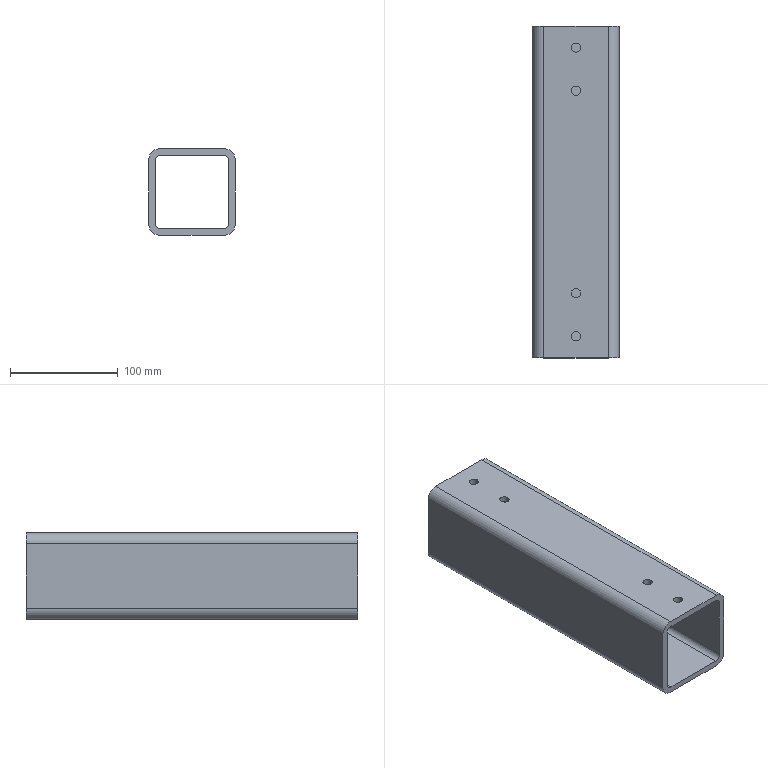Part | SolidWorks | features HoleWzd 3, Fillet 2, Extrusion 1, ICE 1 | 1 solid | 26 faces | box 80 x 307.64 x 80 mm | volume 500055 mm3 | cylinder 16 | plane 10 | commonest cylinder face diameters 8.5 x8 10 x4 20 x4
STEP:
#1=CARTESIAN_POINT('',(0.75,-1.503,34.3));
#2=VERTEX_POINT('',#1);
#3=CARTESIAN_POINT('',(9.25,-1.503,34.3));
#4=VERTEX_POINT('',#3);
#5=CARTESIAN_POINT('',(5.,-1.503,34.3));
#6=DIRECTION('',(0.,0.,1.));
#7=DIRECTION('',(1.,0.,0.));
#8=AXIS2_PLACEMENT_3D('',#5,#6,#7);
#9=CIRCLE('',#8,4.25);
#10=EDGE_CURVE('',#2,#4,#9,.T.);
#11=ORIENTED_EDGE('',*,*,#10,.F.);
#12=CARTESIAN_POINT('',(0.75,-1.503,40.));
#13=VERTEX_POINT('',#12);
#14=CARTESIAN_POINT('',(0.75,-1.503,40.));
#15=DIRECTION('',(0.,0.,1.));
#16=VECTOR('',#15,1000.);
#17=LINE('',#14,#16);
#18=EDGE_CURVE('',#2,#13,#17,.T.);
#19=ORIENTED_EDGE('',*,*,#18,.T.);
#20=CARTESIAN_POINT('',(9.25,-1.503,40.));
#21=VERTEX_POINT('',#20);
#22=CARTESIAN_POINT('',(5.,-1.503,40.));
#23=DIRECTION('',(0.,0.,1.));
#24=DIRECTION('',(1.,0.,0.));
#25=AXIS2_PLACEMENT_3D('',#22,#23,#24);
#26=CIRCLE('',#25,4.25);
#27=EDGE_CURVE('',#13,#21,#26,.T.);
#28=ORIENTED_EDGE('',*,*,#27,.T.);
#29=CARTESIAN_POINT('',(9.25,-1.503,40.));
#30=DIRECTION('',(0.,0.,1.));
#31=VECTOR('',#30,1000.);
#32=LINE('',#29,#31);
#33=EDGE_CURVE('',#4,#21,#32,.T.);
#34=ORIENTED_EDGE('',*,*,#33,.F.);
#35=EDGE_LOOP('',(#11,#19,#28,#34));
#36=FACE_OUTER_BOUND('',#35,.T.);
#37=CARTESIAN_POINT('',(5.,-1.503,40.));
#38=DIRECTION('',(0.,0.,1.));
#39=DIRECTION('',(1.,0.,0.));
#40=AXIS2_PLACEMENT_3D('',#37,#38,#39);
#41=CYLINDRICAL_SURFACE('',#40,4.25);
#42=ADVANCED_FACE('',(#36),#41,.F.);
#43=CARTESIAN_POINT('',(0.75,38.497,34.3));
#44=VERTEX_POINT('',#43);
#45=CARTESIAN_POINT('',(9.25,38.497,34.3));
#46=VERTEX_POINT('',#45);
#47=CARTESIAN_POINT('',(5.,38.497,34.3));
#48=DIRECTION('',(0.,0.,1.));
#49=DIRECTION('',(1.,0.,0.));
#50=AXIS2_PLACEMENT_3D('',#47,#48,#49);
#51=CIRCLE('',#50,4.25);
#52=EDGE_CURVE('',#44,#46,#51,.T.);
#53=ORIENTED_EDGE('',*,*,#52,.F.);
#54=CARTESIAN_POINT('',(0.75,38.497,40.));
#55=VERTEX_POINT('',#54);
#56=CARTESIAN_POINT('',(0.75,38.497,40.));
#57=DIRECTION('',(0.,0.,1.));
#58=VECTOR('',#57,1000.);
#59=LINE('',#56,#58);
#60=EDGE_CURVE('',#44,#55,#59,.T.);
#61=ORIENTED_EDGE('',*,*,#60,.T.);
#62=CARTESIAN_POINT('',(9.25,38.497,40.));
#63=VERTEX_POINT('',#62);
#64=CARTESIAN_POINT('',(5.,38.497,40.));
#65=DIRECTION('',(0.,0.,1.));
#66=DIRECTION('',(1.,0.,0.));
#67=AXIS2_PLACEMENT_3D('',#64,#65,#66);
#68=CIRCLE('',#67,4.25);
#69=EDGE_CURVE('',#55,#63,#68,.T.);
#70=ORIENTED_EDGE('',*,*,#69,.T.);
#71=CARTESIAN_POINT('',(9.25,38.497,40.));
#72=DIRECTION('',(0.,0.,1.));
#73=VECTOR('',#72,1000.);
#74=LINE('',#71,#73);
#75=EDGE_CURVE('',#46,#63,#74,.T.);
#76=ORIENTED_EDGE('',*,*,#75,.F.);
#77=EDGE_LOOP('',(#53,#61,#70,#76));
#78=FACE_OUTER_BOUND('',#77,.T.);
#79=CARTESIAN_POINT('',(5.,38.497,40.));
#80=DIRECTION('',(0.,0.,1.));
#81=DIRECTION('',(1.,0.,0.));
#82=AXIS2_PLACEMENT_3D('',#79,#80,#81);
#83=CYLINDRICAL_SURFACE('',#82,4.25);
#84=ADVANCED_FACE('',(#78),#83,.F.);
#85=CARTESIAN_POINT('',(0.75,-189.143,34.3));
#86=VERTEX_POINT('',#85);
#87=CARTESIAN_POINT('',(9.25,-189.143,34.3));
#88=VERTEX_POINT('',#87);
#89=CARTESIAN_POINT('',(5.,-189.143,34.3));
#90=DIRECTION('',(0.,0.,1.));
#91=DIRECTION('',(1.,0.,0.));
#92=AXIS2_PLACEMENT_3D('',#89,#90,#91);
#93=CIRCLE('',#92,4.25);
#94=EDGE_CURVE('',#86,#88,#93,.T.);
#95=ORIENTED_EDGE('',*,*,#94,.F.);
#96=CARTESIAN_POINT('',(0.75,-189.143,40.));
#97=VERTEX_POINT('',#96);
#98=CARTESIAN_POINT('',(0.75,-189.143,40.));
#99=DIRECTION('',(0.,0.,1.));
#100=VECTOR('',#99,1000.);
#101=LINE('',#98,#100);
#102=EDGE_CURVE('',#86,#97,#101,.T.);
#103=ORIENTED_EDGE('',*,*,#102,.T.);
#104=CARTESIAN_POINT('',(9.25,-189.143,40.));
#105=VERTEX_POINT('',#104);
#106=CARTESIAN_POINT('',(5.,-189.143,40.));
#107=DIRECTION('',(0.,0.,1.));
#108=DIRECTION('',(1.,0.,0.));
#109=AXIS2_PLACEMENT_3D('',#106,#107,#108);
#110=CIRCLE('',#109,4.25);
#111=EDGE_CURVE('',#97,#105,#110,.T.);
#112=ORIENTED_EDGE('',*,*,#111,.T.);
#113=CARTESIAN_POINT('',(9.25,-189.143,40.));
#114=DIRECTION('',(0.,0.,1.));
#115=VECTOR('',#114,1000.);
#116=LINE('',#113,#115);
#117=EDGE_CURVE('',#88,#105,#116,.T.);
#118=ORIENTED_EDGE('',*,*,#117,.F.);
#119=EDGE_LOOP('',(#95,#103,#112,#118));
#120=FACE_OUTER_BOUND('',#119,.T.);
#121=CARTESIAN_POINT('',(5.,-189.143,40.));
#122=DIRECTION('',(0.,0.,1.));
#123=DIRECTION('',(1.,0.,0.));
#124=AXIS2_PLACEMENT_3D('',#121,#122,#123);
#125=CYLINDRICAL_SURFACE('',#124,4.25);
#126=ADVANCED_FACE('',(#120),#125,.F.);
#127=CARTESIAN_POINT('',(0.75,-229.143,34.3));
#128=VERTEX_POINT('',#127);
#129=CARTESIAN_POINT('',(9.25,-229.143,34.3));
#130=VERTEX_POINT('',#129);
#131=CARTESIAN_POINT('',(5.,-229.143,34.3));
#132=DIRECTION('',(0.,0.,1.));
#133=DIRECTION('',(1.,0.,0.));
#134=AXIS2_PLACEMENT_3D('',#131,#132,#133);
#135=CIRCLE('',#134,4.25);
#136=EDGE_CURVE('',#128,#130,#135,.T.);
#137=ORIENTED_EDGE('',*,*,#136,.F.);
#138=CARTESIAN_POINT('',(0.75,-229.143,40.));
#139=VERTEX_POINT('',#138);
#140=CARTESIAN_POINT('',(0.75,-229.143,40.));
#141=DIRECTION('',(0.,0.,1.));
#142=VECTOR('',#141,1000.);
#143=LINE('',#140,#142);
#144=EDGE_CURVE('',#128,#139,#143,.T.);
#145=ORIENTED_EDGE('',*,*,#144,.T.);
#146=CARTESIAN_POINT('',(9.25,-229.143,40.));
#147=VERTEX_POINT('',#146);
#148=CARTESIAN_POINT('',(5.,-229.143,40.));
#149=DIRECTION('',(0.,0.,1.));
#150=DIRECTION('',(1.,0.,0.));
#151=AXIS2_PLACEMENT_3D('',#148,#149,#150);
#152=CIRCLE('',#151,4.25);
#153=EDGE_CURVE('',#139,#147,#152,.T.);
#154=ORIENTED_EDGE('',*,*,#153,.T.);
#155=CARTESIAN_POINT('',(9.25,-229.143,40.));
#156=DIRECTION('',(0.,0.,1.));
#157=VECTOR('',#156,1000.);
#158=LINE('',#155,#157);
#159=EDGE_CURVE('',#130,#147,#158,.T.);
#160=ORIENTED_EDGE('',*,*,#159,.F.);
#161=EDGE_LOOP('',(#137,#145,#154,#160));
#162=FACE_OUTER_BOUND('',#161,.T.);
#163=CARTESIAN_POINT('',(5.,-229.143,40.));
#164=DIRECTION('',(0.,0.,1.));
#165=DIRECTION('',(1.,0.,0.));
#166=AXIS2_PLACEMENT_3D('',#163,#164,#165);
#167=CYLINDRICAL_SURFACE('',#166,4.25);
#168=ADVANCED_FACE('',(#162),#167,.F.);
#169=CARTESIAN_POINT('',(35.,-249.143,-40.));
#170=VERTEX_POINT('',#169);
#171=CARTESIAN_POINT('',(-25.,-249.143,-40.));
#172=VERTEX_POINT('',#171);
#173=CARTESIAN_POINT('',(45.,-249.143,-40.));
#174=DIRECTION('',(-1.,0.,0.));
#175=VECTOR('',#174,1000.);
#176=LINE('',#173,#175);
#177=EDGE_CURVE('',#170,#172,#176,.T.);
#178=ORIENTED_EDGE('',*,*,#177,.T.);
#179=CARTESIAN_POINT('',(-25.,58.497,-40.));
#180=VERTEX_POINT('',#179);
#181=CARTESIAN_POINT('',(-25.,58.497,-40.));
#182=DIRECTION('',(0.,1.,0.));
#183=VECTOR('',#182,1000.);
#184=LINE('',#181,#183);
#185=EDGE_CURVE('',#172,#180,#184,.T.);
#186=ORIENTED_EDGE('',*,*,#185,.T.);
#187=CARTESIAN_POINT('',(35.,58.497,-40.));
#188=VERTEX_POINT('',#187);
#189=CARTESIAN_POINT('',(45.,58.497,-40.));
#190=DIRECTION('',(-1.,0.,0.));
#191=VECTOR('',#190,1000.);
#192=LINE('',#189,#191);
#193=EDGE_CURVE('',#188,#180,#192,.T.);
#194=ORIENTED_EDGE('',*,*,#193,.F.);
#195=CARTESIAN_POINT('',(35.,-249.143,-40.));
#196=DIRECTION('',(0.,-1.,0.));
#197=VECTOR('',#196,1000.);
#198=LINE('',#195,#197);
#199=EDGE_CURVE('',#188,#170,#198,.T.);
#200=ORIENTED_EDGE('',*,*,#199,.T.);
#201=EDGE_LOOP('',(#178,#186,#194,#200));
#202=FACE_OUTER_BOUND('',#201,.T.);
#203=CARTESIAN_POINT('',(45.,58.497,-40.));
#204=DIRECTION('',(0.,0.,-1.));
#205=DIRECTION('',(-1.,0.,0.));
#206=AXIS2_PLACEMENT_3D('',#203,#204,#205);
#207=PLANE('',#206);
#208=ADVANCED_FACE('',(#202),#207,.T.);
#209=CARTESIAN_POINT('',(34.3,58.497,34.3));
#210=VERTEX_POINT('',#209);
#211=CARTESIAN_POINT('',(-24.3,58.497,34.3));
#212=VERTEX_POINT('',#211);
#213=CARTESIAN_POINT('',(39.3,58.497,34.3));
#214=DIRECTION('',(-1.,0.,0.));
#215=VECTOR('',#214,1000.);
#216=LINE('',#213,#215);
#217=EDGE_CURVE('',#210,#212,#216,.T.);
#218=ORIENTED_EDGE('',*,*,#217,.T.);
#219=CARTESIAN_POINT('',(-29.3,58.497,29.3));
#220=VERTEX_POINT('',#219);
#221=CARTESIAN_POINT('',(-24.3,58.497,29.3));
#222=DIRECTION('',(0.,-1.,0.));
#223=DIRECTION('',(0.,0.,1.));
#224=AXIS2_PLACEMENT_3D('',#221,#222,#223);
#225=CIRCLE('',#224,5.);
#226=EDGE_CURVE('',#212,#220,#225,.T.);
#227=ORIENTED_EDGE('',*,*,#226,.T.);
#228=CARTESIAN_POINT('',(-29.3,58.497,-29.3));
#229=VERTEX_POINT('',#228);
#230=CARTESIAN_POINT('',(-29.3,58.497,34.3));
#231=DIRECTION('',(0.,0.,-1.));
#232=VECTOR('',#231,1000.);
#233=LINE('',#230,#232);
#234=EDGE_CURVE('',#220,#229,#233,.T.);
#235=ORIENTED_EDGE('',*,*,#234,.T.);
#236=CARTESIAN_POINT('',(-24.3,58.497,-34.3));
#237=VERTEX_POINT('',#236);
#238=CARTESIAN_POINT('',(-24.3,58.497,-29.3));
#239=DIRECTION('',(0.,-1.,0.));
#240=DIRECTION('',(0.,0.,1.));
#241=AXIS2_PLACEMENT_3D('',#238,#239,#240);
#242=CIRCLE('',#241,5.);
#243=EDGE_CURVE('',#229,#237,#242,.T.);
#244=ORIENTED_EDGE('',*,*,#243,.T.);
#245=CARTESIAN_POINT('',(34.3,58.497,-34.3));
#246=VERTEX_POINT('',#245);
#247=CARTESIAN_POINT('',(-29.3,58.497,-34.3));
#248=DIRECTION('',(1.,0.,0.));
#249=VECTOR('',#248,1000.);
#250=LINE('',#247,#249);
#251=EDGE_CURVE('',#237,#246,#250,.T.);
#252=ORIENTED_EDGE('',*,*,#251,.T.);
#253=CARTESIAN_POINT('',(39.3,58.497,-29.3));
#254=VERTEX_POINT('',#253);
#255=CARTESIAN_POINT('',(34.3,58.497,-29.3));
#256=DIRECTION('',(0.,-1.,0.));
#257=DIRECTION('',(0.,0.,1.));
#258=AXIS2_PLACEMENT_3D('',#255,#256,#257);
#259=CIRCLE('',#258,5.);
#260=EDGE_CURVE('',#246,#254,#259,.T.);
#261=ORIENTED_EDGE('',*,*,#260,.T.);
#262=CARTESIAN_POINT('',(39.3,58.497,29.3));
#263=VERTEX_POINT('',#262);
#264=CARTESIAN_POINT('',(39.3,58.497,-34.3));
#265=DIRECTION('',(0.,0.,1.));
#266=VECTOR('',#265,1000.);
#267=LINE('',#264,#266);
#268=EDGE_CURVE('',#254,#263,#267,.T.);
#269=ORIENTED_EDGE('',*,*,#268,.T.);
#270=CARTESIAN_POINT('',(34.3,58.497,29.3));
#271=DIRECTION('',(0.,-1.,0.));
#272=DIRECTION('',(0.,0.,1.));
#273=AXIS2_PLACEMENT_3D('',#270,#271,#272);
#274=CIRCLE('',#273,5.);
#275=EDGE_CURVE('',#263,#210,#274,.T.);
#276=ORIENTED_EDGE('',*,*,#275,.T.);
#277=EDGE_LOOP('',(#218,#227,#235,#244,#252,#261,#269,#276));
#278=FACE_BOUND('',#277,.T.);
#279=CARTESIAN_POINT('',(-35.,58.497,30.));
#280=VERTEX_POINT('',#279);
#281=CARTESIAN_POINT('',(-35.,58.497,-30.));
#282=VERTEX_POINT('',#281);
#283=CARTESIAN_POINT('',(-35.,58.497,40.));
#284=DIRECTION('',(0.,0.,-1.));
#285=VECTOR('',#284,1000.);
#286=LINE('',#283,#285);
#287=EDGE_CURVE('',#280,#282,#286,.T.);
#288=ORIENTED_EDGE('',*,*,#287,.F.);
#289=CARTESIAN_POINT('',(-25.,58.497,40.));
#290=VERTEX_POINT('',#289);
#291=CARTESIAN_POINT('',(-25.,58.497,30.));
#292=DIRECTION('',(0.,1.,0.));
#293=DIRECTION('',(0.,0.,1.));
#294=AXIS2_PLACEMENT_3D('',#291,#292,#293);
#295=CIRCLE('',#294,10.);
#296=EDGE_CURVE('',#280,#290,#295,.T.);
#297=ORIENTED_EDGE('',*,*,#296,.T.);
#298=CARTESIAN_POINT('',(35.,58.497,40.));
#299=VERTEX_POINT('',#298);
#300=CARTESIAN_POINT('',(45.,58.497,40.));
#301=DIRECTION('',(-1.,0.,0.));
#302=VECTOR('',#301,1000.);
#303=LINE('',#300,#302);
#304=EDGE_CURVE('',#299,#290,#303,.T.);
#305=ORIENTED_EDGE('',*,*,#304,.F.);
#306=CARTESIAN_POINT('',(45.,58.497,30.));
#307=VERTEX_POINT('',#306);
#308=CARTESIAN_POINT('',(35.,58.497,30.));
#309=DIRECTION('',(0.,1.,0.));
#310=DIRECTION('',(0.,0.,1.));
#311=AXIS2_PLACEMENT_3D('',#308,#309,#310);
#312=CIRCLE('',#311,10.);
#313=EDGE_CURVE('',#299,#307,#312,.T.);
#314=ORIENTED_EDGE('',*,*,#313,.T.);
#315=CARTESIAN_POINT('',(45.,58.497,-30.));
#316=VERTEX_POINT('',#315);
#317=CARTESIAN_POINT('',(45.,58.497,40.));
#318=DIRECTION('',(0.,0.,-1.));
#319=VECTOR('',#318,1000.);
#320=LINE('',#317,#319);
#321=EDGE_CURVE('',#307,#316,#320,.T.);
#322=ORIENTED_EDGE('',*,*,#321,.T.);
#323=CARTESIAN_POINT('',(35.,58.497,-30.));
#324=DIRECTION('',(0.,1.,0.));
#325=DIRECTION('',(0.,0.,1.));
#326=AXIS2_PLACEMENT_3D('',#323,#324,#325);
#327=CIRCLE('',#326,10.);
#328=EDGE_CURVE('',#316,#188,#327,.T.);
#329=ORIENTED_EDGE('',*,*,#328,.T.);
#330=ORIENTED_EDGE('',*,*,#193,.T.);
#331=CARTESIAN_POINT('',(-25.,58.497,-30.));
#332=DIRECTION('',(0.,1.,0.));
#333=DIRECTION('',(0.,0.,1.));
#334=AXIS2_PLACEMENT_3D('',#331,#332,#333);
#335=CIRCLE('',#334,10.);
#336=EDGE_CURVE('',#180,#282,#335,.T.);
#337=ORIENTED_EDGE('',*,*,#336,.T.);
#338=EDGE_LOOP('',(#288,#297,#305,#314,#322,#329,#330,#337));
#339=FACE_OUTER_BOUND('',#338,.T.);
#340=CARTESIAN_POINT('',(45.,58.497,40.));
#341=DIRECTION('',(0.,1.,0.));
#342=DIRECTION('',(0.,0.,1.));
#343=AXIS2_PLACEMENT_3D('',#340,#341,#342);
#344=PLANE('',#343);
#345=ADVANCED_FACE('',(#278,#339),#344,.T.);
#346=CARTESIAN_POINT('',(5.,-1.503,40.));
#347=DIRECTION('',(0.,0.,1.));
#348=DIRECTION('',(1.,0.,0.));
#349=AXIS2_PLACEMENT_3D('',#346,#347,#348);
#350=CIRCLE('',#349,4.25);
#351=EDGE_CURVE('',#21,#13,#350,.T.);
#352=ORIENTED_EDGE('',*,*,#351,.F.);
#353=ORIENTED_EDGE('',*,*,#27,.F.);
#354=EDGE_LOOP('',(#352,#353));
#355=FACE_BOUND('',#354,.T.);
#356=CARTESIAN_POINT('',(5.,38.497,40.));
#357=DIRECTION('',(0.,0.,1.));
#358=DIRECTION('',(1.,0.,0.));
#359=AXIS2_PLACEMENT_3D('',#356,#357,#358);
#360=CIRCLE('',#359,4.25);
#361=EDGE_CURVE('',#63,#55,#360,.T.);
#362=ORIENTED_EDGE('',*,*,#361,.F.);
#363=ORIENTED_EDGE('',*,*,#69,.F.);
#364=EDGE_LOOP('',(#362,#363));
#365=FACE_BOUND('',#364,.T.);
#366=CARTESIAN_POINT('',(5.,-189.143,40.));
#367=DIRECTION('',(0.,0.,1.));
#368=DIRECTION('',(1.,0.,0.));
#369=AXIS2_PLACEMENT_3D('',#366,#367,#368);
#370=CIRCLE('',#369,4.25);
#371=EDGE_CURVE('',#105,#97,#370,.T.);
#372=ORIENTED_EDGE('',*,*,#371,.F.);
#373=ORIENTED_EDGE('',*,*,#111,.F.);
#374=EDGE_LOOP('',(#372,#373));
#375=FACE_BOUND('',#374,.T.);
#376=CARTESIAN_POINT('',(5.,-229.143,40.));
#377=DIRECTION('',(0.,0.,1.));
#378=DIRECTION('',(1.,0.,0.));
#379=AXIS2_PLACEMENT_3D('',#376,#377,#378);
#380=CIRCLE('',#379,4.25);
#381=EDGE_CURVE('',#147,#139,#380,.T.);
#382=ORIENTED_EDGE('',*,*,#381,.F.);
#383=ORIENTED_EDGE('',*,*,#153,.F.);
#384=EDGE_LOOP('',(#382,#383));
#385=FACE_BOUND('',#384,.T.);
#386=ORIENTED_EDGE('',*,*,#304,.T.);
#387=CARTESIAN_POINT('',(-25.,-249.143,40.));
#388=VERTEX_POINT('',#387);
#389=CARTESIAN_POINT('',(-25.,-249.143,40.));
#390=DIRECTION('',(0.,-1.,0.));
#391=VECTOR('',#390,1000.);
#392=LINE('',#389,#391);
#393=EDGE_CURVE('',#290,#388,#392,.T.);
#394=ORIENTED_EDGE('',*,*,#393,.T.);
#395=CARTESIAN_POINT('',(35.,-249.143,40.));
#396=VERTEX_POINT('',#395);
#397=CARTESIAN_POINT('',(45.,-249.143,40.));
#398=DIRECTION('',(-1.,0.,0.));
#399=VECTOR('',#398,1000.);
#400=LINE('',#397,#399);
#401=EDGE_CURVE('',#396,#388,#400,.T.);
#402=ORIENTED_EDGE('',*,*,#401,.F.);
#403=CARTESIAN_POINT('',(35.,58.497,40.));
#404=DIRECTION('',(0.,1.,0.));
#405=VECTOR('',#404,1000.);
#406=LINE('',#403,#405);
#407=EDGE_CURVE('',#396,#299,#406,.T.);
#408=ORIENTED_EDGE('',*,*,#407,.T.);
#409=EDGE_LOOP('',(#386,#394,#402,#408));
#410=FACE_OUTER_BOUND('',#409,.T.);
#411=CARTESIAN_POINT('',(45.,-249.143,40.));
#412=DIRECTION('',(0.,0.,1.));
#413=DIRECTION('',(0.,-1.,0.));
#414=AXIS2_PLACEMENT_3D('',#411,#412,#413);
#415=PLANE('',#414);
#416=ADVANCED_FACE('',(#355,#365,#375,#385,#410),#415,.T.);
#417=CARTESIAN_POINT('',(-29.3,-249.143,29.3));
#418=VERTEX_POINT('',#417);
#419=CARTESIAN_POINT('',(-29.3,-249.143,-29.3));
#420=VERTEX_POINT('',#419);
#421=CARTESIAN_POINT('',(-29.3,-249.143,34.3));
#422=DIRECTION('',(0.,0.,-1.));
#423=VECTOR('',#422,1000.);
#424=LINE('',#421,#423);
#425=EDGE_CURVE('',#418,#420,#424,.T.);
#426=ORIENTED_EDGE('',*,*,#425,.F.);
#427=CARTESIAN_POINT('',(-24.3,-249.143,34.3));
#428=VERTEX_POINT('',#427);
#429=CARTESIAN_POINT('',(-24.3,-249.143,29.3));
#430=DIRECTION('',(0.,1.,0.));
#431=DIRECTION('',(0.,0.,-1.));
#432=AXIS2_PLACEMENT_3D('',#429,#430,#431);
#433=CIRCLE('',#432,5.);
#434=EDGE_CURVE('',#418,#428,#433,.T.);
#435=ORIENTED_EDGE('',*,*,#434,.T.);
#436=CARTESIAN_POINT('',(34.3,-249.143,34.3));
#437=VERTEX_POINT('',#436);
#438=CARTESIAN_POINT('',(39.3,-249.143,34.3));
#439=DIRECTION('',(-1.,0.,0.));
#440=VECTOR('',#439,1000.);
#441=LINE('',#438,#440);
#442=EDGE_CURVE('',#437,#428,#441,.T.);
#443=ORIENTED_EDGE('',*,*,#442,.F.);
#444=CARTESIAN_POINT('',(39.3,-249.143,29.3));
#445=VERTEX_POINT('',#444);
#446=CARTESIAN_POINT('',(34.3,-249.143,29.3));
#447=DIRECTION('',(0.,1.,0.));
#448=DIRECTION('',(0.,0.,-1.));
#449=AXIS2_PLACEMENT_3D('',#446,#447,#448);
#450=CIRCLE('',#449,5.);
#451=EDGE_CURVE('',#437,#445,#450,.T.);
#452=ORIENTED_EDGE('',*,*,#451,.T.);
#453=CARTESIAN_POINT('',(39.3,-249.143,-29.3));
#454=VERTEX_POINT('',#453);
#455=CARTESIAN_POINT('',(39.3,-249.143,-34.3));
#456=DIRECTION('',(0.,0.,1.));
#457=VECTOR('',#456,1000.);
#458=LINE('',#455,#457);
#459=EDGE_CURVE('',#454,#445,#458,.T.);
#460=ORIENTED_EDGE('',*,*,#459,.F.);
#461=CARTESIAN_POINT('',(34.3,-249.143,-34.3));
#462=VERTEX_POINT('',#461);
#463=CARTESIAN_POINT('',(34.3,-249.143,-29.3));
#464=DIRECTION('',(0.,1.,0.));
#465=DIRECTION('',(0.,0.,-1.));
#466=AXIS2_PLACEMENT_3D('',#463,#464,#465);
#467=CIRCLE('',#466,5.);
#468=EDGE_CURVE('',#454,#462,#467,.T.);
#469=ORIENTED_EDGE('',*,*,#468,.T.);
#470=CARTESIAN_POINT('',(-24.3,-249.143,-34.3));
#471=VERTEX_POINT('',#470);
#472=CARTESIAN_POINT('',(-29.3,-249.143,-34.3));
#473=DIRECTION('',(1.,0.,0.));
#474=VECTOR('',#473,1000.);
#475=LINE('',#472,#474);
#476=EDGE_CURVE('',#471,#462,#475,.T.);
#477=ORIENTED_EDGE('',*,*,#476,.F.);
#478=CARTESIAN_POINT('',(-24.3,-249.143,-29.3));
#479=DIRECTION('',(0.,1.,0.));
#480=DIRECTION('',(0.,0.,-1.));
#481=AXIS2_PLACEMENT_3D('',#478,#479,#480);
#482=CIRCLE('',#481,5.);
#483=EDGE_CURVE('',#471,#420,#482,.T.);
#484=ORIENTED_EDGE('',*,*,#483,.T.);
#485=EDGE_LOOP('',(#426,#435,#443,#452,#460,#469,#477,#484));
#486=FACE_BOUND('',#485,.T.);
#487=ORIENTED_EDGE('',*,*,#401,.T.);
#488=CARTESIAN_POINT('',(-35.,-249.143,30.));
#489=VERTEX_POINT('',#488);
#490=CARTESIAN_POINT('',(-25.,-249.143,30.));
#491=DIRECTION('',(0.,-1.,0.));
#492=DIRECTION('',(0.,0.,-1.));
#493=AXIS2_PLACEMENT_3D('',#490,#491,#492);
#494=CIRCLE('',#493,10.);
#495=EDGE_CURVE('',#388,#489,#494,.T.);
#496=ORIENTED_EDGE('',*,*,#495,.T.);
#497=CARTESIAN_POINT('',(-35.,-249.143,-30.));
#498=VERTEX_POINT('',#497);
#499=CARTESIAN_POINT('',(-35.,-249.143,-40.));
#500=DIRECTION('',(0.,0.,1.));
#501=VECTOR('',#500,1000.);
#502=LINE('',#499,#501);
#503=EDGE_CURVE('',#498,#489,#502,.T.);
#504=ORIENTED_EDGE('',*,*,#503,.F.);
#505=CARTESIAN_POINT('',(-25.,-249.143,-30.));
#506=DIRECTION('',(0.,-1.,0.));
#507=DIRECTION('',(0.,0.,-1.));
#508=AXIS2_PLACEMENT_3D('',#505,#506,#507);
#509=CIRCLE('',#508,10.);
#510=EDGE_CURVE('',#498,#172,#509,.T.);
#511=ORIENTED_EDGE('',*,*,#510,.T.);
#512=ORIENTED_EDGE('',*,*,#177,.F.);
#513=CARTESIAN_POINT('',(45.,-249.143,-30.));
#514=VERTEX_POINT('',#513);
#515=CARTESIAN_POINT('',(35.,-249.143,-30.));
#516=DIRECTION('',(0.,-1.,0.));
#517=DIRECTION('',(0.,0.,-1.));
#518=AXIS2_PLACEMENT_3D('',#515,#516,#517);
#519=CIRCLE('',#518,10.);
#520=EDGE_CURVE('',#170,#514,#519,.T.);
#521=ORIENTED_EDGE('',*,*,#520,.T.);
#522=CARTESIAN_POINT('',(45.,-249.143,30.));
#523=VERTEX_POINT('',#522);
#524=CARTESIAN_POINT('',(45.,-249.143,-40.));
#525=DIRECTION('',(0.,0.,1.));
#526=VECTOR('',#525,1000.);
#527=LINE('',#524,#526);
#528=EDGE_CURVE('',#514,#523,#527,.T.);
#529=ORIENTED_EDGE('',*,*,#528,.T.);
#530=CARTESIAN_POINT('',(35.,-249.143,30.));
#531=DIRECTION('',(0.,-1.,0.));
#532=DIRECTION('',(0.,0.,-1.));
#533=AXIS2_PLACEMENT_3D('',#530,#531,#532);
#534=CIRCLE('',#533,10.);
#535=EDGE_CURVE('',#523,#396,#534,.T.);
#536=ORIENTED_EDGE('',*,*,#535,.T.);
#537=EDGE_LOOP('',(#487,#496,#504,#511,#512,#521,#529,#536));
#538=FACE_OUTER_BOUND('',#537,.T.);
#539=CARTESIAN_POINT('',(45.,-249.143,-40.));
#540=DIRECTION('',(0.,-1.,0.));
#541=DIRECTION('',(0.,0.,-1.));
#542=AXIS2_PLACEMENT_3D('',#539,#540,#541);
#543=PLANE('',#542);
#544=ADVANCED_FACE('',(#486,#538),#543,.T.);
#545=ORIENTED_EDGE('',*,*,#321,.F.);
#546=CARTESIAN_POINT('',(45.,-249.143,30.));
#547=DIRECTION('',(0.,-1.,0.));
#548=VECTOR('',#547,1000.);
#549=LINE('',#546,#548);
#550=EDGE_CURVE('',#307,#523,#549,.T.);
#551=ORIENTED_EDGE('',*,*,#550,.T.);
#552=ORIENTED_EDGE('',*,*,#528,.F.);
#553=CARTESIAN_POINT('',(45.,58.497,-30.));
#554=DIRECTION('',(0.,1.,0.));
#555=VECTOR('',#554,1000.);
#556=LINE('',#553,#555);
#557=EDGE_CURVE('',#514,#316,#556,.T.);
#558=ORIENTED_EDGE('',*,*,#557,.T.);
#559=EDGE_LOOP('',(#545,#551,#552,#558));
#560=FACE_OUTER_BOUND('',#559,.T.);
#561=CARTESIAN_POINT('',(45.,0.,0.));
#562=DIRECTION('',(-1.,0.,0.));
#563=DIRECTION('',(0.,0.,1.));
#564=AXIS2_PLACEMENT_3D('',#561,#562,#563);
#565=PLANE('',#564);
#566=ADVANCED_FACE('',(#560),#565,.F.);
#567=ORIENTED_EDGE('',*,*,#503,.T.);
#568=CARTESIAN_POINT('',(-35.,0.,30.));
#569=DIRECTION('',(0.,1.,0.));
#570=VECTOR('',#569,1000.);
#571=LINE('',#568,#570);
#572=EDGE_CURVE('',#489,#280,#571,.T.);
#573=ORIENTED_EDGE('',*,*,#572,.T.);
#574=ORIENTED_EDGE('',*,*,#287,.T.);
#575=CARTESIAN_POINT('',(-35.,0.,-30.));
#576=DIRECTION('',(0.,-1.,0.));
#577=VECTOR('',#576,1000.);
#578=LINE('',#575,#577);
#579=EDGE_CURVE('',#282,#498,#578,.T.);
#580=ORIENTED_EDGE('',*,*,#579,.T.);
#581=EDGE_LOOP('',(#567,#573,#574,#580));
#582=FACE_OUTER_BOUND('',#581,.T.);
#583=CARTESIAN_POINT('',(-35.,0.,0.));
#584=DIRECTION('',(-1.,0.,0.));
#585=DIRECTION('',(0.,0.,1.));
#586=AXIS2_PLACEMENT_3D('',#583,#584,#585);
#587=PLANE('',#586);
#588=ADVANCED_FACE('',(#582),#587,.T.);
#589=ORIENTED_EDGE('',*,*,#234,.F.);
#590=CARTESIAN_POINT('',(-29.3,-249.143,29.3));
#591=DIRECTION('',(0.,-1.,0.));
#592=VECTOR('',#591,1000.);
#593=LINE('',#590,#592);
#594=EDGE_CURVE('',#220,#418,#593,.T.);
#595=ORIENTED_EDGE('',*,*,#594,.T.);
#596=ORIENTED_EDGE('',*,*,#425,.T.);
#597=CARTESIAN_POINT('',(-29.3,58.497,-29.3));
#598=DIRECTION('',(0.,1.,0.));
#599=VECTOR('',#598,1000.);
#600=LINE('',#597,#599);
#601=EDGE_CURVE('',#420,#229,#600,.T.);
#602=ORIENTED_EDGE('',*,*,#601,.T.);
#603=EDGE_LOOP('',(#589,#595,#596,#602));
#604=FACE_OUTER_BOUND('',#603,.T.);
#605=CARTESIAN_POINT('',(-29.3,58.497,34.3));
#606=DIRECTION('',(-1.,0.,0.));
#607=DIRECTION('',(0.,0.,1.));
#608=AXIS2_PLACEMENT_3D('',#605,#606,#607);
#609=PLANE('',#608);
#610=ADVANCED_FACE('',(#604),#609,.F.);
#611=CARTESIAN_POINT('',(5.,-1.503,34.3));
#612=DIRECTION('',(0.,0.,1.));
#613=DIRECTION('',(1.,0.,0.));
#614=AXIS2_PLACEMENT_3D('',#611,#612,#613);
#615=CIRCLE('',#614,4.25);
#616=EDGE_CURVE('',#4,#2,#615,.T.);
#617=ORIENTED_EDGE('',*,*,#616,.T.);
#618=ORIENTED_EDGE('',*,*,#10,.T.);
#619=EDGE_LOOP('',(#617,#618));
#620=FACE_BOUND('',#619,.T.);
#621=CARTESIAN_POINT('',(5.,38.497,34.3));
#622=DIRECTION('',(0.,0.,1.));
#623=DIRECTION('',(1.,0.,0.));
#624=AXIS2_PLACEMENT_3D('',#621,#622,#623);
#625=CIRCLE('',#624,4.25);
#626=EDGE_CURVE('',#46,#44,#625,.T.);
#627=ORIENTED_EDGE('',*,*,#626,.T.);
#628=ORIENTED_EDGE('',*,*,#52,.T.);
#629=EDGE_LOOP('',(#627,#628));
#630=FACE_BOUND('',#629,.T.);
#631=CARTESIAN_POINT('',(5.,-189.143,34.3));
#632=DIRECTION('',(0.,0.,1.));
#633=DIRECTION('',(1.,0.,0.));
#634=AXIS2_PLACEMENT_3D('',#631,#632,#633);
#635=CIRCLE('',#634,4.25);
#636=EDGE_CURVE('',#88,#86,#635,.T.);
#637=ORIENTED_EDGE('',*,*,#636,.T.);
#638=ORIENTED_EDGE('',*,*,#94,.T.);
#639=EDGE_LOOP('',(#637,#638));
#640=FACE_BOUND('',#639,.T.);
#641=CARTESIAN_POINT('',(5.,-229.143,34.3));
#642=DIRECTION('',(0.,0.,1.));
#643=DIRECTION('',(1.,0.,0.));
#644=AXIS2_PLACEMENT_3D('',#641,#642,#643);
#645=CIRCLE('',#644,4.25);
#646=EDGE_CURVE('',#130,#128,#645,.T.);
#647=ORIENTED_EDGE('',*,*,#646,.T.);
#648=ORIENTED_EDGE('',*,*,#136,.T.);
#649=EDGE_LOOP('',(#647,#648));
#650=FACE_BOUND('',#649,.T.);
#651=ORIENTED_EDGE('',*,*,#217,.F.);
#652=CARTESIAN_POINT('',(34.3,-249.143,34.3));
#653=DIRECTION('',(0.,-1.,0.));
#654=VECTOR('',#653,1000.);
#655=LINE('',#652,#654);
#656=EDGE_CURVE('',#210,#437,#655,.T.);
#657=ORIENTED_EDGE('',*,*,#656,.T.);
#658=ORIENTED_EDGE('',*,*,#442,.T.);
#659=CARTESIAN_POINT('',(-24.3,58.497,34.3));
#660=DIRECTION('',(0.,1.,0.));
#661=VECTOR('',#660,1000.);
#662=LINE('',#659,#661);
#663=EDGE_CURVE('',#428,#212,#662,.T.);
#664=ORIENTED_EDGE('',*,*,#663,.T.);
#665=EDGE_LOOP('',(#651,#657,#658,#664));
#666=FACE_OUTER_BOUND('',#665,.T.);
#667=CARTESIAN_POINT('',(39.3,58.497,34.3));
#668=DIRECTION('',(0.,0.,1.));
#669=DIRECTION('',(1.,0.,0.));
#670=AXIS2_PLACEMENT_3D('',#667,#668,#669);
#671=PLANE('',#670);
#672=ADVANCED_FACE('',(#620,#630,#640,#650,#666),#671,.F.);
#673=ORIENTED_EDGE('',*,*,#459,.T.);
#674=CARTESIAN_POINT('',(39.3,58.497,29.3));
#675=DIRECTION('',(0.,1.,0.));
#676=VECTOR('',#675,1000.);
#677=LINE('',#674,#676);
#678=EDGE_CURVE('',#445,#263,#677,.T.);
#679=ORIENTED_EDGE('',*,*,#678,.T.);
#680=ORIENTED_EDGE('',*,*,#268,.F.);
#681=CARTESIAN_POINT('',(39.3,-249.143,-29.3));
#682=DIRECTION('',(0.,-1.,0.));
#683=VECTOR('',#682,1000.);
#684=LINE('',#681,#683);
#685=EDGE_CURVE('',#254,#454,#684,.T.);
#686=ORIENTED_EDGE('',*,*,#685,.T.);
#687=EDGE_LOOP('',(#673,#679,#680,#686));
#688=FACE_OUTER_BOUND('',#687,.T.);
#689=CARTESIAN_POINT('',(39.3,58.497,-34.3));
#690=DIRECTION('',(1.,0.,0.));
#691=DIRECTION('',(0.,0.,-1.));
#692=AXIS2_PLACEMENT_3D('',#689,#690,#691);
#693=PLANE('',#692);
#694=ADVANCED_FACE('',(#688),#693,.F.);
#695=ORIENTED_EDGE('',*,*,#476,.T.);
#696=CARTESIAN_POINT('',(34.3,58.497,-34.3));
#697=DIRECTION('',(0.,1.,0.));
#698=VECTOR('',#697,1000.);
#699=LINE('',#696,#698);
#700=EDGE_CURVE('',#462,#246,#699,.T.);
#701=ORIENTED_EDGE('',*,*,#700,.T.);
#702=ORIENTED_EDGE('',*,*,#251,.F.);
#703=CARTESIAN_POINT('',(-24.3,-249.143,-34.3));
#704=DIRECTION('',(0.,-1.,0.));
#705=VECTOR('',#704,1000.);
#706=LINE('',#703,#705);
#707=EDGE_CURVE('',#237,#471,#706,.T.);
#708=ORIENTED_EDGE('',*,*,#707,.T.);
#709=EDGE_LOOP('',(#695,#701,#702,#708));
#710=FACE_OUTER_BOUND('',#709,.T.);
#711=CARTESIAN_POINT('',(-29.3,58.497,-34.3));
#712=DIRECTION('',(0.,0.,-1.));
#713=DIRECTION('',(-1.,0.,0.));
#714=AXIS2_PLACEMENT_3D('',#711,#712,#713);
#715=PLANE('',#714);
#716=ADVANCED_FACE('',(#710),#715,.F.);
#717=ORIENTED_EDGE('',*,*,#144,.F.);
#718=ORIENTED_EDGE('',*,*,#646,.F.);
#719=ORIENTED_EDGE('',*,*,#159,.T.);
#720=ORIENTED_EDGE('',*,*,#381,.T.);
#721=EDGE_LOOP('',(#717,#718,#719,#720));
#722=FACE_OUTER_BOUND('',#721,.T.);
#723=CARTESIAN_POINT('',(5.,-229.143,40.));
#724=DIRECTION('',(0.,0.,1.));
#725=DIRECTION('',(1.,0.,0.));
#726=AXIS2_PLACEMENT_3D('',#723,#724,#725);
#727=CYLINDRICAL_SURFACE('',#726,4.25);
#728=ADVANCED_FACE('',(#722),#727,.F.);
#729=ORIENTED_EDGE('',*,*,#102,.F.);
#730=ORIENTED_EDGE('',*,*,#636,.F.);
#731=ORIENTED_EDGE('',*,*,#117,.T.);
#732=ORIENTED_EDGE('',*,*,#371,.T.);
#733=EDGE_LOOP('',(#729,#730,#731,#732));
#734=FACE_OUTER_BOUND('',#733,.T.);
#735=CARTESIAN_POINT('',(5.,-189.143,40.));
#736=DIRECTION('',(0.,0.,1.));
#737=DIRECTION('',(1.,0.,0.));
#738=AXIS2_PLACEMENT_3D('',#735,#736,#737);
#739=CYLINDRICAL_SURFACE('',#738,4.25);
#740=ADVANCED_FACE('',(#734),#739,.F.);
#741=ORIENTED_EDGE('',*,*,#275,.F.);
#742=ORIENTED_EDGE('',*,*,#678,.F.);
#743=ORIENTED_EDGE('',*,*,#451,.F.);
#744=ORIENTED_EDGE('',*,*,#656,.F.);
#745=EDGE_LOOP('',(#741,#742,#743,#744));
#746=FACE_OUTER_BOUND('',#745,.T.);
#747=CARTESIAN_POINT('',(34.3,58.497,29.3));
#748=DIRECTION('',(0.,1.,0.));
#749=DIRECTION('',(0.,0.,1.));
#750=AXIS2_PLACEMENT_3D('',#747,#748,#749);
#751=CYLINDRICAL_SURFACE('',#750,5.);
#752=ADVANCED_FACE('',(#746),#751,.F.);
#753=ORIENTED_EDGE('',*,*,#226,.F.);
#754=ORIENTED_EDGE('',*,*,#663,.F.);
#755=ORIENTED_EDGE('',*,*,#434,.F.);
#756=ORIENTED_EDGE('',*,*,#594,.F.);
#757=EDGE_LOOP('',(#753,#754,#755,#756));
#758=FACE_OUTER_BOUND('',#757,.T.);
#759=CARTESIAN_POINT('',(-24.3,58.497,29.3));
#760=DIRECTION('',(0.,1.,0.));
#761=DIRECTION('',(0.,0.,1.));
#762=AXIS2_PLACEMENT_3D('',#759,#760,#761);
#763=CYLINDRICAL_SURFACE('',#762,5.);
#764=ADVANCED_FACE('',(#758),#763,.F.);
#765=ORIENTED_EDGE('',*,*,#260,.F.);
#766=ORIENTED_EDGE('',*,*,#700,.F.);
#767=ORIENTED_EDGE('',*,*,#468,.F.);
#768=ORIENTED_EDGE('',*,*,#685,.F.);
#769=EDGE_LOOP('',(#765,#766,#767,#768));
#770=FACE_OUTER_BOUND('',#769,.T.);
#771=CARTESIAN_POINT('',(34.3,58.497,-29.3));
#772=DIRECTION('',(0.,1.,0.));
#773=DIRECTION('',(0.,0.,1.));
#774=AXIS2_PLACEMENT_3D('',#771,#772,#773);
#775=CYLINDRICAL_SURFACE('',#774,5.);
#776=ADVANCED_FACE('',(#770),#775,.F.);
#777=ORIENTED_EDGE('',*,*,#243,.F.);
#778=ORIENTED_EDGE('',*,*,#601,.F.);
#779=ORIENTED_EDGE('',*,*,#483,.F.);
#780=ORIENTED_EDGE('',*,*,#707,.F.);
#781=EDGE_LOOP('',(#777,#778,#779,#780));
#782=FACE_OUTER_BOUND('',#781,.T.);
#783=CARTESIAN_POINT('',(-24.3,58.497,-29.3));
#784=DIRECTION('',(0.,1.,0.));
#785=DIRECTION('',(0.,0.,1.));
#786=AXIS2_PLACEMENT_3D('',#783,#784,#785);
#787=CYLINDRICAL_SURFACE('',#786,5.);
#788=ADVANCED_FACE('',(#782),#787,.F.);
#789=ORIENTED_EDGE('',*,*,#495,.F.);
#790=ORIENTED_EDGE('',*,*,#393,.F.);
#791=ORIENTED_EDGE('',*,*,#296,.F.);
#792=ORIENTED_EDGE('',*,*,#572,.F.);
#793=EDGE_LOOP('',(#789,#790,#791,#792));
#794=FACE_OUTER_BOUND('',#793,.T.);
#795=CARTESIAN_POINT('',(-25.,0.,30.));
#796=DIRECTION('',(0.,1.,0.));
#797=DIRECTION('',(0.,0.,1.));
#798=AXIS2_PLACEMENT_3D('',#795,#796,#797);
#799=CYLINDRICAL_SURFACE('',#798,10.);
#800=ADVANCED_FACE('',(#794),#799,.T.);
#801=ORIENTED_EDGE('',*,*,#336,.F.);
#802=ORIENTED_EDGE('',*,*,#185,.F.);
#803=ORIENTED_EDGE('',*,*,#510,.F.);
#804=ORIENTED_EDGE('',*,*,#579,.F.);
#805=EDGE_LOOP('',(#801,#802,#803,#804));
#806=FACE_OUTER_BOUND('',#805,.T.);
#807=CARTESIAN_POINT('',(-25.,0.,-30.));
#808=DIRECTION('',(0.,-1.,0.));
#809=DIRECTION('',(0.,0.,-1.));
#810=AXIS2_PLACEMENT_3D('',#807,#808,#809);
#811=CYLINDRICAL_SURFACE('',#810,10.);
#812=ADVANCED_FACE('',(#806),#811,.T.);
#813=ORIENTED_EDGE('',*,*,#535,.F.);
#814=ORIENTED_EDGE('',*,*,#550,.F.);
#815=ORIENTED_EDGE('',*,*,#313,.F.);
#816=ORIENTED_EDGE('',*,*,#407,.F.);
#817=EDGE_LOOP('',(#813,#814,#815,#816));
#818=FACE_OUTER_BOUND('',#817,.T.);
#819=CARTESIAN_POINT('',(35.,-249.143,30.));
#820=DIRECTION('',(0.,-1.,0.));
#821=DIRECTION('',(0.,0.,-1.));
#822=AXIS2_PLACEMENT_3D('',#819,#820,#821);
#823=CYLINDRICAL_SURFACE('',#822,10.);
#824=ADVANCED_FACE('',(#818),#823,.T.);
#825=ORIENTED_EDGE('',*,*,#328,.F.);
#826=ORIENTED_EDGE('',*,*,#557,.F.);
#827=ORIENTED_EDGE('',*,*,#520,.F.);
#828=ORIENTED_EDGE('',*,*,#199,.F.);
#829=EDGE_LOOP('',(#825,#826,#827,#828));
#830=FACE_OUTER_BOUND('',#829,.T.);
#831=CARTESIAN_POINT('',(35.,58.497,-30.));
#832=DIRECTION('',(0.,1.,0.));
#833=DIRECTION('',(0.,0.,1.));
#834=AXIS2_PLACEMENT_3D('',#831,#832,#833);
#835=CYLINDRICAL_SURFACE('',#834,10.);
#836=ADVANCED_FACE('',(#830),#835,.T.);
#837=ORIENTED_EDGE('',*,*,#60,.F.);
#838=ORIENTED_EDGE('',*,*,#626,.F.);
#839=ORIENTED_EDGE('',*,*,#75,.T.);
#840=ORIENTED_EDGE('',*,*,#361,.T.);
#841=EDGE_LOOP('',(#837,#838,#839,#840));
#842=FACE_OUTER_BOUND('',#841,.T.);
#843=CARTESIAN_POINT('',(5.,38.497,40.));
#844=DIRECTION('',(0.,0.,1.));
#845=DIRECTION('',(1.,0.,0.));
#846=AXIS2_PLACEMENT_3D('',#843,#844,#845);
#847=CYLINDRICAL_SURFACE('',#846,4.25);
#848=ADVANCED_FACE('',(#842),#847,.F.);
#849=ORIENTED_EDGE('',*,*,#18,.F.);
#850=ORIENTED_EDGE('',*,*,#616,.F.);
#851=ORIENTED_EDGE('',*,*,#33,.T.);
#852=ORIENTED_EDGE('',*,*,#351,.T.);
#853=EDGE_LOOP('',(#849,#850,#851,#852));
#854=FACE_OUTER_BOUND('',#853,.T.);
#855=CARTESIAN_POINT('',(5.,-1.503,40.));
#856=DIRECTION('',(0.,0.,1.));
#857=DIRECTION('',(1.,0.,0.));
#858=AXIS2_PLACEMENT_3D('',#855,#856,#857);
#859=CYLINDRICAL_SURFACE('',#858,4.25);
#860=ADVANCED_FACE('',(#854),#859,.F.);
#861=CLOSED_SHELL('',(#42,#84,#126,#168,#208,#345,#416,#544,#566,#588,#610,#672,#694,#716,#728,#740,#752,#764,#776,#788,#800,#812,#824,#836,#848,#860));
#862=MANIFOLD_SOLID_BREP('',#861);
#863=CARTESIAN_POINT('',(0.,0.,0.));
#864=DIRECTION('',(0.,0.,1.));
#865=DIRECTION('',(1.,0.,0.));
#866=AXIS2_PLACEMENT_3D('',#863,#864,#865);
#867=(LENGTH_UNIT()NAMED_UNIT(*)SI_UNIT(.MILLI.,.METRE.));
#868=UNCERTAINTY_MEASURE_WITH_UNIT(LENGTH_MEASURE(0.00001),#867,'','');
#869=(NAMED_UNIT(*)PLANE_ANGLE_UNIT()SI_UNIT($,.RADIAN.));
#870=(NAMED_UNIT(*)SI_UNIT($,.STERADIAN.)SOLID_ANGLE_UNIT());
#871=(GEOMETRIC_REPRESENTATION_CONTEXT(3)GLOBAL_UNCERTAINTY_ASSIGNED_CONTEXT((#868))GLOBAL_UNIT_ASSIGNED_CONTEXT((#867,#869,#870))REPRESENTATION_CONTEXT('',''));
#872=ADVANCED_BREP_SHAPE_REPRESENTATION('',(#862,#866),#871);